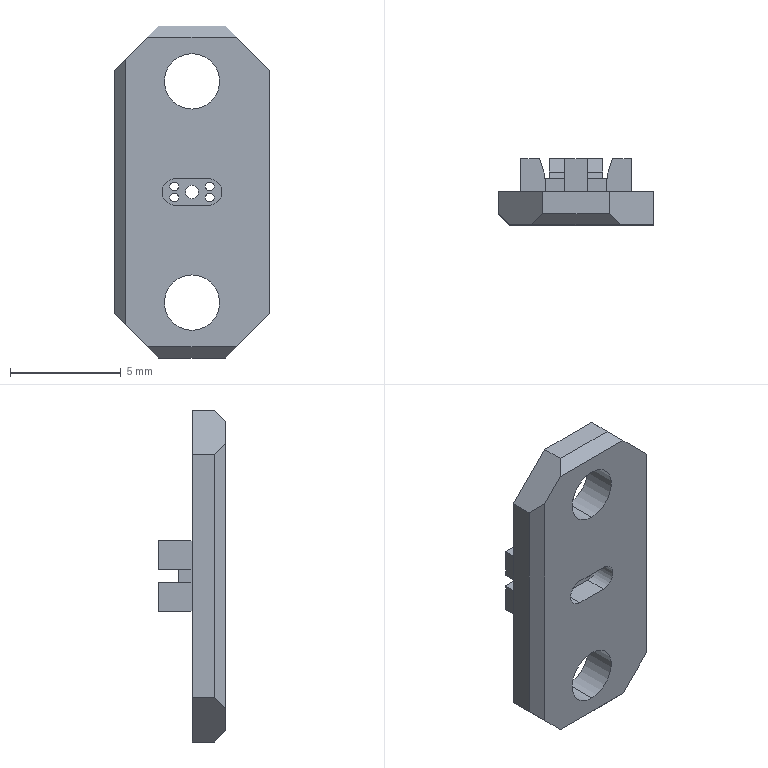Part | SolidWorks | features ICE 14, Chamfer 5, Extrusion 1 | 1 solid | 85 faces | box 7 x 3 x 15 mm | volume 138.292 mm3 | plane 67 | cylinder 18 | commonest cylinder face diameters 0.4 x8 2.5 x4 0.6 x2 0.95 x2 1.2 x2